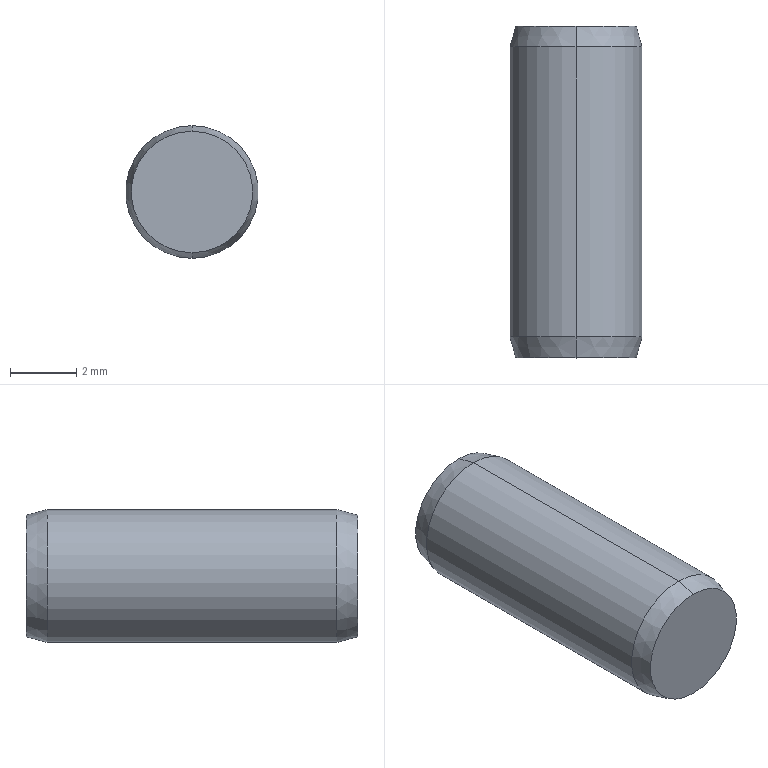Part | STEP file | Cylindrical pin 4x10-C1 | 1 solid | 8 faces | box 4 x 10 x 4 mm | volume 124.365 mm3 | cone 4 | cylinder 2 | plane 2 | commonest cylinder face diameters 4 x2
STEP:
#1=CARTESIAN_POINT('',(0.,0.,0.));
#2=DIRECTION('',(0.,0.,1.));
#3=DIRECTION('',(1.,0.,0.));
#4=AXIS2_PLACEMENT_3D('',#1,#2,#3);
#5=CARTESIAN_POINT('',(0.,-5.,-1.831));
#6=VERTEX_POINT('',#5);
#7=CARTESIAN_POINT('',(0.,-5.,1.831));
#8=VERTEX_POINT('',#7);
#9=CARTESIAN_POINT('',(0.,-5.,0.));
#10=DIRECTION('',(0.,-1.,0.));
#11=DIRECTION('',(0.,0.,-1.));
#12=AXIS2_PLACEMENT_3D('',#9,#10,#11);
#13=CIRCLE('',#12,1.831);
#14=CARTESIAN_POINT('',(0.,-4.37,0.));
#15=DIRECTION('',(0.,1.,0.));
#16=DIRECTION('',(0.,0.,1.));
#17=AXIS2_PLACEMENT_3D('',#14,#15,#16);
#18=CONICAL_SURFACE('',#17,2.,0.2618);
#19=CARTESIAN_POINT('',(3.142,-0.63));
#20=DIRECTION('',(-1.,0.));
#21=VECTOR('',#20,1.);
#22=LINE('',#19,#21);
#23=(GEOMETRIC_REPRESENTATION_CONTEXT(2)PARAMETRIC_REPRESENTATION_CONTEXT()REPRESENTATION_CONTEXT('',''));
#24=DEFINITIONAL_REPRESENTATION('',(#22),#23);
#25=PCURVE('',#18,#24);
#26=CARTESIAN_POINT('',(0.,-5.,0.));
#27=DIRECTION('',(0.,-1.,0.));
#28=DIRECTION('',(0.,0.,-1.));
#29=AXIS2_PLACEMENT_3D('',#26,#27,#28);
#30=PLANE('',#29);
#31=CARTESIAN_POINT('',(0.,0.));
#32=DIRECTION('',(1.,0.));
#33=AXIS2_PLACEMENT_2D('',#31,#32);
#34=CIRCLE('',#33,1.831);
#35=(GEOMETRIC_REPRESENTATION_CONTEXT(2)PARAMETRIC_REPRESENTATION_CONTEXT()REPRESENTATION_CONTEXT('',''));
#36=DEFINITIONAL_REPRESENTATION('',(#34),#35);
#37=PCURVE('',#30,#36);
#38=SURFACE_CURVE('',#13,(#25,#37),.PCURVE_S1.);
#39=EDGE_CURVE('',#6,#8,#38,.T.);
#40=ORIENTED_EDGE('',*,*,#39,.F.);
#41=CARTESIAN_POINT('',(0.,-4.37,-2.));
#42=VERTEX_POINT('',#41);
#43=CARTESIAN_POINT('',(0.,-4.37,-2.));
#44=DIRECTION('',(0.,0.9659,-0.2588));
#45=VECTOR('',#44,1.);
#46=LINE('',#43,#45);
#47=CARTESIAN_POINT('',(3.142,0.));
#48=DIRECTION('',(0.,1.));
#49=VECTOR('',#48,1.);
#50=LINE('',#47,#49);
#51=(GEOMETRIC_REPRESENTATION_CONTEXT(2)PARAMETRIC_REPRESENTATION_CONTEXT()REPRESENTATION_CONTEXT('',''));
#52=DEFINITIONAL_REPRESENTATION('',(#50),#51);
#53=PCURVE('',#18,#52);
#54=CARTESIAN_POINT('',(0.,-4.37,0.));
#55=DIRECTION('',(0.,1.,0.));
#56=DIRECTION('',(0.,0.,1.));
#57=AXIS2_PLACEMENT_3D('',#54,#55,#56);
#58=CONICAL_SURFACE('',#57,2.,0.2618);
#59=CARTESIAN_POINT('',(3.142,0.));
#60=DIRECTION('',(0.,1.));
#61=VECTOR('',#60,1.);
#62=LINE('',#59,#61);
#63=(GEOMETRIC_REPRESENTATION_CONTEXT(2)PARAMETRIC_REPRESENTATION_CONTEXT()REPRESENTATION_CONTEXT('',''));
#64=DEFINITIONAL_REPRESENTATION('',(#62),#63);
#65=PCURVE('',#58,#64);
#66=SURFACE_CURVE('',#46,(#53,#65),.PCURVE_S1.);
#67=EDGE_CURVE('',#6,#42,#66,.T.);
#68=ORIENTED_EDGE('',*,*,#67,.T.);
#69=CARTESIAN_POINT('',(0.,-4.37,2.));
#70=VERTEX_POINT('',#69);
#71=CARTESIAN_POINT('',(0.,-4.37,0.));
#72=DIRECTION('',(0.,1.,0.));
#73=DIRECTION('',(0.,0.,-1.));
#74=AXIS2_PLACEMENT_3D('',#71,#72,#73);
#75=CIRCLE('',#74,2.);
#76=CARTESIAN_POINT('',(-3.142,0.));
#77=DIRECTION('',(1.,0.));
#78=VECTOR('',#77,1.);
#79=LINE('',#76,#78);
#80=(GEOMETRIC_REPRESENTATION_CONTEXT(2)PARAMETRIC_REPRESENTATION_CONTEXT()REPRESENTATION_CONTEXT('',''));
#81=DEFINITIONAL_REPRESENTATION('',(#79),#80);
#82=PCURVE('',#18,#81);
#83=CARTESIAN_POINT('',(0.,6.034,0.));
#84=DIRECTION('',(0.,1.,0.));
#85=DIRECTION('',(0.,0.,1.));
#86=AXIS2_PLACEMENT_3D('',#83,#84,#85);
#87=CYLINDRICAL_SURFACE('',#86,2.);
#88=CARTESIAN_POINT('',(-3.142,-10.404));
#89=DIRECTION('',(1.,0.));
#90=VECTOR('',#89,1.);
#91=LINE('',#88,#90);
#92=(GEOMETRIC_REPRESENTATION_CONTEXT(2)PARAMETRIC_REPRESENTATION_CONTEXT()REPRESENTATION_CONTEXT('',''));
#93=DEFINITIONAL_REPRESENTATION('',(#91),#92);
#94=PCURVE('',#87,#93);
#95=SURFACE_CURVE('',#75,(#82,#94),.PCURVE_S1.);
#96=EDGE_CURVE('',#70,#42,#95,.T.);
#97=ORIENTED_EDGE('',*,*,#96,.F.);
#98=CARTESIAN_POINT('',(0.,-4.37,2.));
#99=DIRECTION('',(0.,0.9659,0.2588));
#100=VECTOR('',#99,1.);
#101=LINE('',#98,#100);
#102=CARTESIAN_POINT('',(0.,0.));
#103=DIRECTION('',(0.,1.));
#104=VECTOR('',#103,1.);
#105=LINE('',#102,#104);
#106=(GEOMETRIC_REPRESENTATION_CONTEXT(2)PARAMETRIC_REPRESENTATION_CONTEXT()REPRESENTATION_CONTEXT('',''));
#107=DEFINITIONAL_REPRESENTATION('',(#105),#106);
#108=PCURVE('',#18,#107);
#109=CARTESIAN_POINT('',(6.283,0.));
#110=DIRECTION('',(0.,1.));
#111=VECTOR('',#110,1.);
#112=LINE('',#109,#111);
#113=(GEOMETRIC_REPRESENTATION_CONTEXT(2)PARAMETRIC_REPRESENTATION_CONTEXT()REPRESENTATION_CONTEXT('',''));
#114=DEFINITIONAL_REPRESENTATION('',(#112),#113);
#115=PCURVE('',#58,#114);
#116=SURFACE_CURVE('',#101,(#108,#115),.PCURVE_S1.);
#117=EDGE_CURVE('',#8,#70,#116,.T.);
#118=ORIENTED_EDGE('',*,*,#117,.F.);
#119=EDGE_LOOP('',(#40,#68,#97,#118));
#120=FACE_BOUND('',#119,.T.);
#121=ADVANCED_FACE('',(#120),#18,.T.);
#122=CARTESIAN_POINT('',(0.,5.,1.831));
#123=VERTEX_POINT('',#122);
#124=CARTESIAN_POINT('',(0.,5.,-1.831));
#125=VERTEX_POINT('',#124);
#126=CARTESIAN_POINT('',(0.,5.,0.));
#127=DIRECTION('',(0.,1.,0.));
#128=DIRECTION('',(0.,0.,1.));
#129=AXIS2_PLACEMENT_3D('',#126,#127,#128);
#130=CIRCLE('',#129,1.831);
#131=CARTESIAN_POINT('',(0.,5.,0.));
#132=DIRECTION('',(0.,-1.,0.));
#133=DIRECTION('',(0.,0.,-1.));
#134=AXIS2_PLACEMENT_3D('',#131,#132,#133);
#135=CONICAL_SURFACE('',#134,1.831,0.2618);
#136=CARTESIAN_POINT('',(3.142,0.));
#137=DIRECTION('',(-1.,0.));
#138=VECTOR('',#137,1.);
#139=LINE('',#136,#138);
#140=(GEOMETRIC_REPRESENTATION_CONTEXT(2)PARAMETRIC_REPRESENTATION_CONTEXT()REPRESENTATION_CONTEXT('',''));
#141=DEFINITIONAL_REPRESENTATION('',(#139),#140);
#142=PCURVE('',#135,#141);
#143=CARTESIAN_POINT('',(0.,5.,0.));
#144=DIRECTION('',(0.,1.,0.));
#145=DIRECTION('',(0.,0.,1.));
#146=AXIS2_PLACEMENT_3D('',#143,#144,#145);
#147=PLANE('',#146);
#148=CARTESIAN_POINT('',(0.,0.));
#149=DIRECTION('',(1.,0.));
#150=AXIS2_PLACEMENT_2D('',#148,#149);
#151=CIRCLE('',#150,1.831);
#152=(GEOMETRIC_REPRESENTATION_CONTEXT(2)PARAMETRIC_REPRESENTATION_CONTEXT()REPRESENTATION_CONTEXT('',''));
#153=DEFINITIONAL_REPRESENTATION('',(#151),#152);
#154=PCURVE('',#147,#153);
#155=SURFACE_CURVE('',#130,(#142,#154),.PCURVE_S1.);
#156=EDGE_CURVE('',#123,#125,#155,.T.);
#157=ORIENTED_EDGE('',*,*,#156,.F.);
#158=CARTESIAN_POINT('',(0.,4.37,2.));
#159=VERTEX_POINT('',#158);
#160=CARTESIAN_POINT('',(0.,5.,1.831));
#161=DIRECTION('',(0.,-0.9659,0.2588));
#162=VECTOR('',#161,1.);
#163=LINE('',#160,#162);
#164=CARTESIAN_POINT('',(3.142,0.));
#165=DIRECTION('',(0.,1.));
#166=VECTOR('',#165,1.);
#167=LINE('',#164,#166);
#168=(GEOMETRIC_REPRESENTATION_CONTEXT(2)PARAMETRIC_REPRESENTATION_CONTEXT()REPRESENTATION_CONTEXT('',''));
#169=DEFINITIONAL_REPRESENTATION('',(#167),#168);
#170=PCURVE('',#135,#169);
#171=CARTESIAN_POINT('',(0.,5.,0.));
#172=DIRECTION('',(0.,-1.,0.));
#173=DIRECTION('',(0.,0.,-1.));
#174=AXIS2_PLACEMENT_3D('',#171,#172,#173);
#175=CONICAL_SURFACE('',#174,1.831,0.2618);
#176=CARTESIAN_POINT('',(3.142,0.));
#177=DIRECTION('',(0.,1.));
#178=VECTOR('',#177,1.);
#179=LINE('',#176,#178);
#180=(GEOMETRIC_REPRESENTATION_CONTEXT(2)PARAMETRIC_REPRESENTATION_CONTEXT()REPRESENTATION_CONTEXT('',''));
#181=DEFINITIONAL_REPRESENTATION('',(#179),#180);
#182=PCURVE('',#175,#181);
#183=SURFACE_CURVE('',#163,(#170,#182),.PCURVE_S1.);
#184=EDGE_CURVE('',#123,#159,#183,.T.);
#185=ORIENTED_EDGE('',*,*,#184,.T.);
#186=CARTESIAN_POINT('',(0.,4.37,-2.));
#187=VERTEX_POINT('',#186);
#188=CARTESIAN_POINT('',(0.,4.37,0.));
#189=DIRECTION('',(0.,-1.,0.));
#190=DIRECTION('',(0.,0.,1.));
#191=AXIS2_PLACEMENT_3D('',#188,#189,#190);
#192=CIRCLE('',#191,2.);
#193=CARTESIAN_POINT('',(-3.142,0.63));
#194=DIRECTION('',(1.,0.));
#195=VECTOR('',#194,1.);
#196=LINE('',#193,#195);
#197=(GEOMETRIC_REPRESENTATION_CONTEXT(2)PARAMETRIC_REPRESENTATION_CONTEXT()REPRESENTATION_CONTEXT('',''));
#198=DEFINITIONAL_REPRESENTATION('',(#196),#197);
#199=PCURVE('',#135,#198);
#200=CARTESIAN_POINT('',(6.283,-1.664));
#201=DIRECTION('',(-1.,0.));
#202=VECTOR('',#201,1.);
#203=LINE('',#200,#202);
#204=(GEOMETRIC_REPRESENTATION_CONTEXT(2)PARAMETRIC_REPRESENTATION_CONTEXT()REPRESENTATION_CONTEXT('',''));
#205=DEFINITIONAL_REPRESENTATION('',(#203),#204);
#206=PCURVE('',#87,#205);
#207=SURFACE_CURVE('',#192,(#199,#206),.PCURVE_S1.);
#208=EDGE_CURVE('',#187,#159,#207,.T.);
#209=ORIENTED_EDGE('',*,*,#208,.F.);
#210=CARTESIAN_POINT('',(0.,5.,-1.831));
#211=DIRECTION('',(0.,-0.9659,-0.2588));
#212=VECTOR('',#211,1.);
#213=LINE('',#210,#212);
#214=CARTESIAN_POINT('',(0.,0.));
#215=DIRECTION('',(0.,1.));
#216=VECTOR('',#215,1.);
#217=LINE('',#214,#216);
#218=(GEOMETRIC_REPRESENTATION_CONTEXT(2)PARAMETRIC_REPRESENTATION_CONTEXT()REPRESENTATION_CONTEXT('',''));
#219=DEFINITIONAL_REPRESENTATION('',(#217),#218);
#220=PCURVE('',#135,#219);
#221=CARTESIAN_POINT('',(6.283,0.));
#222=DIRECTION('',(0.,1.));
#223=VECTOR('',#222,1.);
#224=LINE('',#221,#223);
#225=(GEOMETRIC_REPRESENTATION_CONTEXT(2)PARAMETRIC_REPRESENTATION_CONTEXT()REPRESENTATION_CONTEXT('',''));
#226=DEFINITIONAL_REPRESENTATION('',(#224),#225);
#227=PCURVE('',#175,#226);
#228=SURFACE_CURVE('',#213,(#220,#227),.PCURVE_S1.);
#229=EDGE_CURVE('',#125,#187,#228,.T.);
#230=ORIENTED_EDGE('',*,*,#229,.F.);
#231=EDGE_LOOP('',(#157,#185,#209,#230));
#232=FACE_BOUND('',#231,.T.);
#233=ADVANCED_FACE('',(#232),#135,.T.);
#234=ORIENTED_EDGE('',*,*,#96,.T.);
#235=CARTESIAN_POINT('',(0.,6.034,-2.));
#236=DIRECTION('',(0.,1.,0.));
#237=VECTOR('',#236,1.);
#238=LINE('',#235,#237);
#239=CARTESIAN_POINT('',(3.142,0.));
#240=DIRECTION('',(0.,1.));
#241=VECTOR('',#240,1.);
#242=LINE('',#239,#241);
#243=(GEOMETRIC_REPRESENTATION_CONTEXT(2)PARAMETRIC_REPRESENTATION_CONTEXT()REPRESENTATION_CONTEXT('',''));
#244=DEFINITIONAL_REPRESENTATION('',(#242),#243);
#245=PCURVE('',#87,#244);
#246=CARTESIAN_POINT('',(0.,6.034,0.));
#247=DIRECTION('',(0.,1.,0.));
#248=DIRECTION('',(0.,0.,1.));
#249=AXIS2_PLACEMENT_3D('',#246,#247,#248);
#250=CYLINDRICAL_SURFACE('',#249,2.);
#251=CARTESIAN_POINT('',(3.142,0.));
#252=DIRECTION('',(0.,1.));
#253=VECTOR('',#252,1.);
#254=LINE('',#251,#253);
#255=(GEOMETRIC_REPRESENTATION_CONTEXT(2)PARAMETRIC_REPRESENTATION_CONTEXT()REPRESENTATION_CONTEXT('',''));
#256=DEFINITIONAL_REPRESENTATION('',(#254),#255);
#257=PCURVE('',#250,#256);
#258=SURFACE_CURVE('',#238,(#245,#257),.PCURVE_S1.);
#259=EDGE_CURVE('',#42,#187,#258,.T.);
#260=ORIENTED_EDGE('',*,*,#259,.T.);
#261=ORIENTED_EDGE('',*,*,#208,.T.);
#262=CARTESIAN_POINT('',(0.,6.034,2.));
#263=DIRECTION('',(0.,1.,0.));
#264=VECTOR('',#263,1.);
#265=LINE('',#262,#264);
#266=CARTESIAN_POINT('',(0.,0.));
#267=DIRECTION('',(0.,1.));
#268=VECTOR('',#267,1.);
#269=LINE('',#266,#268);
#270=(GEOMETRIC_REPRESENTATION_CONTEXT(2)PARAMETRIC_REPRESENTATION_CONTEXT()REPRESENTATION_CONTEXT('',''));
#271=DEFINITIONAL_REPRESENTATION('',(#269),#270);
#272=PCURVE('',#87,#271);
#273=CARTESIAN_POINT('',(6.283,0.));
#274=DIRECTION('',(0.,1.));
#275=VECTOR('',#274,1.);
#276=LINE('',#273,#275);
#277=(GEOMETRIC_REPRESENTATION_CONTEXT(2)PARAMETRIC_REPRESENTATION_CONTEXT()REPRESENTATION_CONTEXT('',''));
#278=DEFINITIONAL_REPRESENTATION('',(#276),#277);
#279=PCURVE('',#250,#278);
#280=SURFACE_CURVE('',#265,(#272,#279),.PCURVE_S1.);
#281=EDGE_CURVE('',#70,#159,#280,.T.);
#282=ORIENTED_EDGE('',*,*,#281,.F.);
#283=EDGE_LOOP('',(#234,#260,#261,#282));
#284=FACE_BOUND('',#283,.T.);
#285=ADVANCED_FACE('',(#284),#87,.T.);
#286=CARTESIAN_POINT('',(0.,-5.,0.));
#287=DIRECTION('',(0.,-1.,0.));
#288=DIRECTION('',(0.,0.,-1.));
#289=AXIS2_PLACEMENT_3D('',#286,#287,#288);
#290=CIRCLE('',#289,1.831);
#291=CARTESIAN_POINT('',(0.,0.));
#292=DIRECTION('',(1.,0.));
#293=AXIS2_PLACEMENT_2D('',#291,#292);
#294=CIRCLE('',#293,1.831);
#295=(GEOMETRIC_REPRESENTATION_CONTEXT(2)PARAMETRIC_REPRESENTATION_CONTEXT()REPRESENTATION_CONTEXT('',''));
#296=DEFINITIONAL_REPRESENTATION('',(#294),#295);
#297=PCURVE('',#30,#296);
#298=CARTESIAN_POINT('',(9.425,-0.63));
#299=DIRECTION('',(-1.,0.));
#300=VECTOR('',#299,1.);
#301=LINE('',#298,#300);
#302=(GEOMETRIC_REPRESENTATION_CONTEXT(2)PARAMETRIC_REPRESENTATION_CONTEXT()REPRESENTATION_CONTEXT('',''));
#303=DEFINITIONAL_REPRESENTATION('',(#301),#302);
#304=PCURVE('',#58,#303);
#305=SURFACE_CURVE('',#290,(#297,#304),.PCURVE_S1.);
#306=EDGE_CURVE('',#8,#6,#305,.T.);
#307=ORIENTED_EDGE('',*,*,#306,.T.);
#308=ORIENTED_EDGE('',*,*,#39,.T.);
#309=EDGE_LOOP('',(#307,#308));
#310=FACE_BOUND('',#309,.T.);
#311=ADVANCED_FACE('',(#310),#30,.T.);
#312=ORIENTED_EDGE('',*,*,#259,.F.);
#313=CARTESIAN_POINT('',(0.,-4.37,0.));
#314=DIRECTION('',(0.,1.,0.));
#315=DIRECTION('',(0.,0.,-1.));
#316=AXIS2_PLACEMENT_3D('',#313,#314,#315);
#317=CIRCLE('',#316,2.);
#318=CARTESIAN_POINT('',(3.142,-10.404));
#319=DIRECTION('',(1.,0.));
#320=VECTOR('',#319,1.);
#321=LINE('',#318,#320);
#322=(GEOMETRIC_REPRESENTATION_CONTEXT(2)PARAMETRIC_REPRESENTATION_CONTEXT()REPRESENTATION_CONTEXT('',''));
#323=DEFINITIONAL_REPRESENTATION('',(#321),#322);
#324=PCURVE('',#250,#323);
#325=CARTESIAN_POINT('',(3.142,0.));
#326=DIRECTION('',(1.,0.));
#327=VECTOR('',#326,1.);
#328=LINE('',#325,#327);
#329=(GEOMETRIC_REPRESENTATION_CONTEXT(2)PARAMETRIC_REPRESENTATION_CONTEXT()REPRESENTATION_CONTEXT('',''));
#330=DEFINITIONAL_REPRESENTATION('',(#328),#329);
#331=PCURVE('',#58,#330);
#332=SURFACE_CURVE('',#317,(#324,#331),.PCURVE_S1.);
#333=EDGE_CURVE('',#42,#70,#332,.T.);
#334=ORIENTED_EDGE('',*,*,#333,.T.);
#335=ORIENTED_EDGE('',*,*,#281,.T.);
#336=CARTESIAN_POINT('',(0.,4.37,0.));
#337=DIRECTION('',(0.,-1.,0.));
#338=DIRECTION('',(0.,0.,1.));
#339=AXIS2_PLACEMENT_3D('',#336,#337,#338);
#340=CIRCLE('',#339,2.);
#341=CARTESIAN_POINT('',(6.283,-1.664));
#342=DIRECTION('',(-1.,0.));
#343=VECTOR('',#342,1.);
#344=LINE('',#341,#343);
#345=(GEOMETRIC_REPRESENTATION_CONTEXT(2)PARAMETRIC_REPRESENTATION_CONTEXT()REPRESENTATION_CONTEXT('',''));
#346=DEFINITIONAL_REPRESENTATION('',(#344),#345);
#347=PCURVE('',#250,#346);
#348=CARTESIAN_POINT('',(3.142,0.63));
#349=DIRECTION('',(1.,0.));
#350=VECTOR('',#349,1.);
#351=LINE('',#348,#350);
#352=(GEOMETRIC_REPRESENTATION_CONTEXT(2)PARAMETRIC_REPRESENTATION_CONTEXT()REPRESENTATION_CONTEXT('',''));
#353=DEFINITIONAL_REPRESENTATION('',(#351),#352);
#354=PCURVE('',#175,#353);
#355=SURFACE_CURVE('',#340,(#347,#354),.PCURVE_S1.);
#356=EDGE_CURVE('',#159,#187,#355,.T.);
#357=ORIENTED_EDGE('',*,*,#356,.T.);
#358=EDGE_LOOP('',(#312,#334,#335,#357));
#359=FACE_BOUND('',#358,.T.);
#360=ADVANCED_FACE('',(#359),#250,.T.);
#361=CARTESIAN_POINT('',(0.,5.,0.));
#362=DIRECTION('',(0.,1.,0.));
#363=DIRECTION('',(0.,0.,1.));
#364=AXIS2_PLACEMENT_3D('',#361,#362,#363);
#365=CIRCLE('',#364,1.831);
#366=CARTESIAN_POINT('',(0.,0.));
#367=DIRECTION('',(1.,0.));
#368=AXIS2_PLACEMENT_2D('',#366,#367);
#369=CIRCLE('',#368,1.831);
#370=(GEOMETRIC_REPRESENTATION_CONTEXT(2)PARAMETRIC_REPRESENTATION_CONTEXT()REPRESENTATION_CONTEXT('',''));
#371=DEFINITIONAL_REPRESENTATION('',(#369),#370);
#372=PCURVE('',#147,#371);
#373=CARTESIAN_POINT('',(9.425,0.));
#374=DIRECTION('',(-1.,0.));
#375=VECTOR('',#374,1.);
#376=LINE('',#373,#375);
#377=(GEOMETRIC_REPRESENTATION_CONTEXT(2)PARAMETRIC_REPRESENTATION_CONTEXT()REPRESENTATION_CONTEXT('',''));
#378=DEFINITIONAL_REPRESENTATION('',(#376),#377);
#379=PCURVE('',#175,#378);
#380=SURFACE_CURVE('',#365,(#372,#379),.PCURVE_S1.);
#381=EDGE_CURVE('',#125,#123,#380,.T.);
#382=ORIENTED_EDGE('',*,*,#381,.T.);
#383=ORIENTED_EDGE('',*,*,#156,.T.);
#384=EDGE_LOOP('',(#382,#383));
#385=FACE_BOUND('',#384,.T.);
#386=ADVANCED_FACE('',(#385),#147,.T.);
#387=ORIENTED_EDGE('',*,*,#184,.F.);
#388=ORIENTED_EDGE('',*,*,#381,.F.);
#389=ORIENTED_EDGE('',*,*,#229,.T.);
#390=ORIENTED_EDGE('',*,*,#356,.F.);
#391=EDGE_LOOP('',(#387,#388,#389,#390));
#392=FACE_BOUND('',#391,.T.);
#393=ADVANCED_FACE('',(#392),#175,.T.);
#394=ORIENTED_EDGE('',*,*,#67,.F.);
#395=ORIENTED_EDGE('',*,*,#306,.F.);
#396=ORIENTED_EDGE('',*,*,#117,.T.);
#397=ORIENTED_EDGE('',*,*,#333,.F.);
#398=EDGE_LOOP('',(#394,#395,#396,#397));
#399=FACE_BOUND('',#398,.T.);
#400=ADVANCED_FACE('',(#399),#58,.T.);
#401=CLOSED_SHELL('',(#121,#233,#285,#311,#360,#386,#393,#400));
#402=MANIFOLD_SOLID_BREP('',#401);
#403=(LENGTH_UNIT()NAMED_UNIT(*)SI_UNIT(.MILLI.,.METRE.));
#404=UNCERTAINTY_MEASURE_WITH_UNIT(LENGTH_MEASURE(0.0000001),#403,'','');
#405=(NAMED_UNIT(*)PLANE_ANGLE_UNIT()SI_UNIT($,.RADIAN.));
#406=(NAMED_UNIT(*)SI_UNIT($,.STERADIAN.)SOLID_ANGLE_UNIT());
#407=(GEOMETRIC_REPRESENTATION_CONTEXT(3)GLOBAL_UNCERTAINTY_ASSIGNED_CONTEXT((#404))GLOBAL_UNIT_ASSIGNED_CONTEXT((#403,#405,#406))REPRESENTATION_CONTEXT('',''));
#408=ADVANCED_BREP_SHAPE_REPRESENTATION('',(#4,#402),#407);